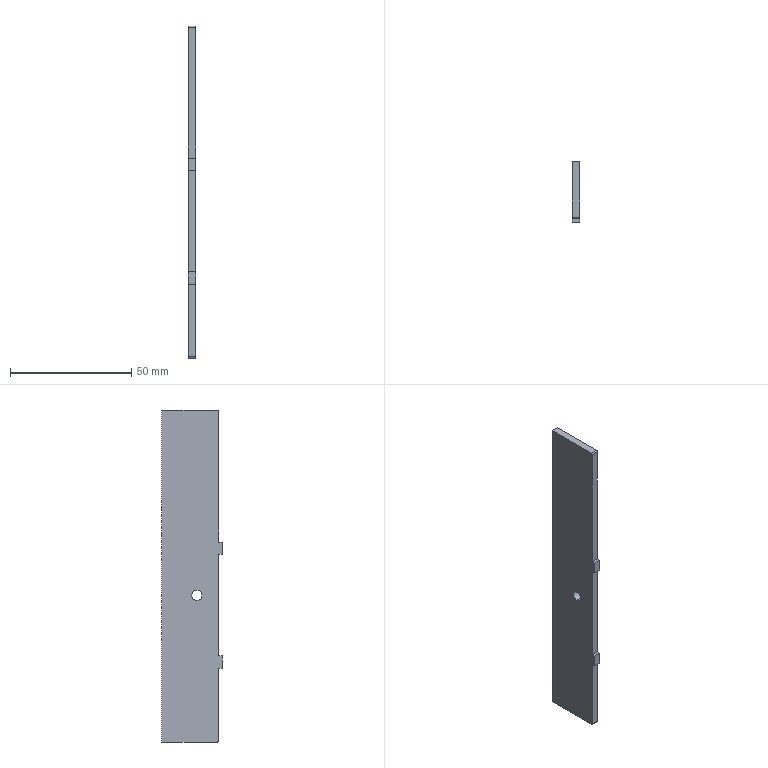Part | STEP file | HESS-408-70-15W-W-23-lower door frame support plate | 1 solid | 18 faces | box 3 x 25 x 137 mm | volume 9662 mm3 | plane 14 | cylinder 4 | commonest cylinder face diameters 1 x2 4.2 x2
STEP:
#1=CARTESIAN_POINT('',(0.,0.,0.));
#2=DIRECTION('',(0.,0.,1.));
#3=DIRECTION('',(1.,0.,0.));
#4=AXIS2_PLACEMENT_3D('',#1,#2,#3);
#5=CARTESIAN_POINT('',(-3.,-2.75,-10.1));
#6=VERTEX_POINT('',#5);
#7=CARTESIAN_POINT('',(0.,-2.75,-10.1));
#8=VERTEX_POINT('',#7);
#9=CARTESIAN_POINT('',(-10.,-2.75,-10.1));
#10=DIRECTION('',(1.,0.,0.));
#11=VECTOR('',#10,1.);
#12=LINE('',#9,#11);
#13=CARTESIAN_POINT('',(-10.,-2.75,-8.));
#14=DIRECTION('',(1.,0.,0.));
#15=DIRECTION('',(0.,0.,-1.));
#16=AXIS2_PLACEMENT_3D('',#13,#14,#15);
#17=CYLINDRICAL_SURFACE('',#16,2.1);
#18=CARTESIAN_POINT('',(6.283,0.));
#19=DIRECTION('',(0.,1.));
#20=VECTOR('',#19,1.);
#21=LINE('',#18,#20);
#22=(GEOMETRIC_REPRESENTATION_CONTEXT(2)PARAMETRIC_REPRESENTATION_CONTEXT()REPRESENTATION_CONTEXT('',''));
#23=DEFINITIONAL_REPRESENTATION('',(#21),#22);
#24=PCURVE('',#17,#23);
#25=CARTESIAN_POINT('',(-10.,-2.75,-8.));
#26=DIRECTION('',(1.,0.,0.));
#27=DIRECTION('',(0.,0.,-1.));
#28=AXIS2_PLACEMENT_3D('',#25,#26,#27);
#29=CYLINDRICAL_SURFACE('',#28,2.1);
#30=CARTESIAN_POINT('',(0.,0.));
#31=DIRECTION('',(0.,1.));
#32=VECTOR('',#31,1.);
#33=LINE('',#30,#32);
#34=(GEOMETRIC_REPRESENTATION_CONTEXT(2)PARAMETRIC_REPRESENTATION_CONTEXT()REPRESENTATION_CONTEXT('',''));
#35=DEFINITIONAL_REPRESENTATION('',(#33),#34);
#36=PCURVE('',#29,#35);
#37=SURFACE_CURVE('',#12,(#24,#36),.PCURVE_S1.);
#38=EDGE_CURVE('',#6,#8,#37,.T.);
#39=ORIENTED_EDGE('',*,*,#38,.T.);
#40=CARTESIAN_POINT('',(0.,-2.75,-5.9));
#41=VERTEX_POINT('',#40);
#42=CARTESIAN_POINT('',(0.,-2.75,-8.));
#43=DIRECTION('',(1.,0.,0.));
#44=DIRECTION('',(0.,0.,-1.));
#45=AXIS2_PLACEMENT_3D('',#42,#43,#44);
#46=CIRCLE('',#45,2.1);
#47=CARTESIAN_POINT('',(0.,10.));
#48=DIRECTION('',(1.,0.));
#49=VECTOR('',#48,1.);
#50=LINE('',#47,#49);
#51=(GEOMETRIC_REPRESENTATION_CONTEXT(2)PARAMETRIC_REPRESENTATION_CONTEXT()REPRESENTATION_CONTEXT('',''));
#52=DEFINITIONAL_REPRESENTATION('',(#50),#51);
#53=PCURVE('',#17,#52);
#54=CARTESIAN_POINT('',(0.,0.,0.));
#55=DIRECTION('',(-1.,0.,0.));
#56=DIRECTION('',(0.,0.,1.));
#57=AXIS2_PLACEMENT_3D('',#54,#55,#56);
#58=PLANE('',#57);
#59=CARTESIAN_POINT('',(-10.1,-2.75));
#60=CARTESIAN_POINT('',(-10.1,0.8873));
#61=CARTESIAN_POINT('',(-6.95,-0.9313));
#62=CARTESIAN_POINT('',(-3.8,-2.75));
#63=CARTESIAN_POINT('',(-6.95,-4.569));
#64=CARTESIAN_POINT('',(-10.1,-6.387));
#65=CARTESIAN_POINT('',(-10.1,-2.75));
#66=(BOUNDED_CURVE()B_SPLINE_CURVE(2,(#59,#60,#61,#62,#63,#64,#65),.UNSPECIFIED.,.T.,.F.)B_SPLINE_CURVE_WITH_KNOTS((1,2,2,2,2,1),(-2.094,0.,2.094,4.189,6.283,8.378),.UNSPECIFIED.)CURVE()GEOMETRIC_REPRESENTATION_ITEM()RATIONAL_B_SPLINE_CURVE((1.,0.5,1.,0.5,1.,0.5,1.))REPRESENTATION_ITEM(''));
#67=(GEOMETRIC_REPRESENTATION_CONTEXT(2)PARAMETRIC_REPRESENTATION_CONTEXT()REPRESENTATION_CONTEXT('',''));
#68=DEFINITIONAL_REPRESENTATION('',(#66),#67);
#69=PCURVE('',#58,#68);
#70=SURFACE_CURVE('',#46,(#53,#69),.PCURVE_S1.);
#71=EDGE_CURVE('',#41,#8,#70,.T.);
#72=ORIENTED_EDGE('',*,*,#71,.F.);
#73=CARTESIAN_POINT('',(-3.,-2.75,-5.9));
#74=VERTEX_POINT('',#73);
#75=CARTESIAN_POINT('',(-10.,-2.75,-5.9));
#76=DIRECTION('',(1.,0.,0.));
#77=VECTOR('',#76,1.);
#78=LINE('',#75,#77);
#79=CARTESIAN_POINT('',(3.142,0.));
#80=DIRECTION('',(0.,1.));
#81=VECTOR('',#80,1.);
#82=LINE('',#79,#81);
#83=(GEOMETRIC_REPRESENTATION_CONTEXT(2)PARAMETRIC_REPRESENTATION_CONTEXT()REPRESENTATION_CONTEXT('',''));
#84=DEFINITIONAL_REPRESENTATION('',(#82),#83);
#85=PCURVE('',#17,#84);
#86=CARTESIAN_POINT('',(3.142,0.));
#87=DIRECTION('',(0.,1.));
#88=VECTOR('',#87,1.);
#89=LINE('',#86,#88);
#90=(GEOMETRIC_REPRESENTATION_CONTEXT(2)PARAMETRIC_REPRESENTATION_CONTEXT()REPRESENTATION_CONTEXT('',''));
#91=DEFINITIONAL_REPRESENTATION('',(#89),#90);
#92=PCURVE('',#29,#91);
#93=SURFACE_CURVE('',#78,(#85,#92),.PCURVE_S1.);
#94=EDGE_CURVE('',#74,#41,#93,.T.);
#95=ORIENTED_EDGE('',*,*,#94,.F.);
#96=CARTESIAN_POINT('',(-3.,-2.75,-8.));
#97=DIRECTION('',(1.,0.,0.));
#98=DIRECTION('',(0.,0.,-1.));
#99=AXIS2_PLACEMENT_3D('',#96,#97,#98);
#100=CIRCLE('',#99,2.1);
#101=CARTESIAN_POINT('',(0.,7.));
#102=DIRECTION('',(1.,0.));
#103=VECTOR('',#102,1.);
#104=LINE('',#101,#103);
#105=(GEOMETRIC_REPRESENTATION_CONTEXT(2)PARAMETRIC_REPRESENTATION_CONTEXT()REPRESENTATION_CONTEXT('',''));
#106=DEFINITIONAL_REPRESENTATION('',(#104),#105);
#107=PCURVE('',#17,#106);
#108=CARTESIAN_POINT('',(-3.,0.,0.));
#109=DIRECTION('',(-1.,0.,0.));
#110=DIRECTION('',(0.,0.,1.));
#111=AXIS2_PLACEMENT_3D('',#108,#109,#110);
#112=PLANE('',#111);
#113=CARTESIAN_POINT('',(-10.1,-2.75));
#114=CARTESIAN_POINT('',(-10.1,0.8873));
#115=CARTESIAN_POINT('',(-6.95,-0.9313));
#116=CARTESIAN_POINT('',(-3.8,-2.75));
#117=CARTESIAN_POINT('',(-6.95,-4.569));
#118=CARTESIAN_POINT('',(-10.1,-6.387));
#119=CARTESIAN_POINT('',(-10.1,-2.75));
#120=(BOUNDED_CURVE()B_SPLINE_CURVE(2,(#113,#114,#115,#116,#117,#118,#119),.UNSPECIFIED.,.T.,.F.)B_SPLINE_CURVE_WITH_KNOTS((1,2,2,2,2,1),(-2.094,0.,2.094,4.189,6.283,8.378),.UNSPECIFIED.)CURVE()GEOMETRIC_REPRESENTATION_ITEM()RATIONAL_B_SPLINE_CURVE((1.,0.5,1.,0.5,1.,0.5,1.))REPRESENTATION_ITEM(''));
#121=(GEOMETRIC_REPRESENTATION_CONTEXT(2)PARAMETRIC_REPRESENTATION_CONTEXT()REPRESENTATION_CONTEXT('',''));
#122=DEFINITIONAL_REPRESENTATION('',(#120),#121);
#123=PCURVE('',#112,#122);
#124=SURFACE_CURVE('',#100,(#107,#123),.PCURVE_S1.);
#125=EDGE_CURVE('',#74,#6,#124,.T.);
#126=ORIENTED_EDGE('',*,*,#125,.T.);
#127=EDGE_LOOP('',(#39,#72,#95,#126));
#128=FACE_BOUND('',#127,.F.);
#129=ADVANCED_FACE('',(#128),#17,.F.);
#130=CARTESIAN_POINT('',(0.,-13.25,14.));
#131=VERTEX_POINT('',#130);
#132=CARTESIAN_POINT('',(0.,-11.75,14.));
#133=VERTEX_POINT('',#132);
#134=CARTESIAN_POINT('',(0.,-11.75,14.));
#135=DIRECTION('',(0.,1.,0.));
#136=VECTOR('',#135,1.);
#137=LINE('',#134,#136);
#138=CARTESIAN_POINT('',(14.,-11.75));
#139=DIRECTION('',(0.,1.));
#140=VECTOR('',#139,1.);
#141=LINE('',#138,#140);
#142=(GEOMETRIC_REPRESENTATION_CONTEXT(2)PARAMETRIC_REPRESENTATION_CONTEXT()REPRESENTATION_CONTEXT('',''));
#143=DEFINITIONAL_REPRESENTATION('',(#141),#142);
#144=PCURVE('',#58,#143);
#145=CARTESIAN_POINT('',(0.,-11.75,14.));
#146=DIRECTION('',(0.,0.,1.));
#147=DIRECTION('',(1.,0.,0.));
#148=AXIS2_PLACEMENT_3D('',#145,#146,#147);
#149=PLANE('',#148);
#150=CARTESIAN_POINT('',(0.,0.));
#151=DIRECTION('',(0.,1.));
#152=VECTOR('',#151,1.);
#153=LINE('',#150,#152);
#154=(GEOMETRIC_REPRESENTATION_CONTEXT(2)PARAMETRIC_REPRESENTATION_CONTEXT()REPRESENTATION_CONTEXT('',''));
#155=DEFINITIONAL_REPRESENTATION('',(#153),#154);
#156=PCURVE('',#149,#155);
#157=SURFACE_CURVE('',#137,(#144,#156),.PCURVE_S1.);
#158=EDGE_CURVE('',#131,#133,#157,.T.);
#159=ORIENTED_EDGE('',*,*,#158,.F.);
#160=CARTESIAN_POINT('',(0.,-13.25,9.));
#161=VERTEX_POINT('',#160);
#162=CARTESIAN_POINT('',(0.,-13.25,0.));
#163=DIRECTION('',(0.,0.,1.));
#164=VECTOR('',#163,1.);
#165=LINE('',#162,#164);
#166=CARTESIAN_POINT('',(0.,-13.25));
#167=DIRECTION('',(1.,0.));
#168=VECTOR('',#167,1.);
#169=LINE('',#166,#168);
#170=(GEOMETRIC_REPRESENTATION_CONTEXT(2)PARAMETRIC_REPRESENTATION_CONTEXT()REPRESENTATION_CONTEXT('',''));
#171=DEFINITIONAL_REPRESENTATION('',(#169),#170);
#172=PCURVE('',#58,#171);
#173=CARTESIAN_POINT('',(0.,-13.25,9.));
#174=DIRECTION('',(0.,-1.,0.));
#175=DIRECTION('',(0.,0.,-1.));
#176=AXIS2_PLACEMENT_3D('',#173,#174,#175);
#177=PLANE('',#176);
#178=CARTESIAN_POINT('',(9.,0.));
#179=DIRECTION('',(-1.,0.));
#180=VECTOR('',#179,1.);
#181=LINE('',#178,#180);
#182=(GEOMETRIC_REPRESENTATION_CONTEXT(2)PARAMETRIC_REPRESENTATION_CONTEXT()REPRESENTATION_CONTEXT('',''));
#183=DEFINITIONAL_REPRESENTATION('',(#181),#182);
#184=PCURVE('',#177,#183);
#185=SURFACE_CURVE('',#165,(#172,#184),.PCURVE_S1.);
#186=EDGE_CURVE('',#161,#131,#185,.T.);
#187=ORIENTED_EDGE('',*,*,#186,.F.);
#188=CARTESIAN_POINT('',(0.,-11.75,9.));
#189=VERTEX_POINT('',#188);
#190=CARTESIAN_POINT('',(0.,-11.75,9.));
#191=DIRECTION('',(0.,-1.,0.));
#192=VECTOR('',#191,1.);
#193=LINE('',#190,#192);
#194=CARTESIAN_POINT('',(9.,-11.75));
#195=DIRECTION('',(0.,-1.));
#196=VECTOR('',#195,1.);
#197=LINE('',#194,#196);
#198=(GEOMETRIC_REPRESENTATION_CONTEXT(2)PARAMETRIC_REPRESENTATION_CONTEXT()REPRESENTATION_CONTEXT('',''));
#199=DEFINITIONAL_REPRESENTATION('',(#197),#198);
#200=PCURVE('',#58,#199);
#201=CARTESIAN_POINT('',(0.,-11.75,9.));
#202=DIRECTION('',(0.,0.,-1.));
#203=DIRECTION('',(-1.,0.,0.));
#204=AXIS2_PLACEMENT_3D('',#201,#202,#203);
#205=PLANE('',#204);
#206=CARTESIAN_POINT('',(0.,0.));
#207=DIRECTION('',(0.,-1.));
#208=VECTOR('',#207,1.);
#209=LINE('',#206,#208);
#210=(GEOMETRIC_REPRESENTATION_CONTEXT(2)PARAMETRIC_REPRESENTATION_CONTEXT()REPRESENTATION_CONTEXT('',''));
#211=DEFINITIONAL_REPRESENTATION('',(#209),#210);
#212=PCURVE('',#205,#211);
#213=SURFACE_CURVE('',#193,(#200,#212),.PCURVE_S1.);
#214=EDGE_CURVE('',#189,#161,#213,.T.);
#215=ORIENTED_EDGE('',*,*,#214,.F.);
#216=CARTESIAN_POINT('',(0.,-11.75,-33.));
#217=VERTEX_POINT('',#216);
#218=CARTESIAN_POINT('',(0.,-11.75,0.));
#219=DIRECTION('',(0.,0.,1.));
#220=VECTOR('',#219,1.);
#221=LINE('',#218,#220);
#222=CARTESIAN_POINT('',(0.,-11.75));
#223=DIRECTION('',(1.,0.));
#224=VECTOR('',#223,1.);
#225=LINE('',#222,#224);
#226=(GEOMETRIC_REPRESENTATION_CONTEXT(2)PARAMETRIC_REPRESENTATION_CONTEXT()REPRESENTATION_CONTEXT('',''));
#227=DEFINITIONAL_REPRESENTATION('',(#225),#226);
#228=PCURVE('',#58,#227);
#229=CARTESIAN_POINT('',(-3.,-11.75,68.5));
#230=DIRECTION('',(0.,-1.,0.));
#231=DIRECTION('',(0.,0.,-1.));
#232=AXIS2_PLACEMENT_3D('',#229,#230,#231);
#233=PLANE('',#232);
#234=CARTESIAN_POINT('',(68.5,3.));
#235=DIRECTION('',(-1.,0.));
#236=VECTOR('',#235,1.);
#237=LINE('',#234,#236);
#238=(GEOMETRIC_REPRESENTATION_CONTEXT(2)PARAMETRIC_REPRESENTATION_CONTEXT()REPRESENTATION_CONTEXT('',''));
#239=DEFINITIONAL_REPRESENTATION('',(#237),#238);
#240=PCURVE('',#233,#239);
#241=SURFACE_CURVE('',#221,(#228,#240),.PCURVE_S1.);
#242=EDGE_CURVE('',#217,#189,#241,.T.);
#243=ORIENTED_EDGE('',*,*,#242,.F.);
#244=CARTESIAN_POINT('',(0.,-13.25,-33.));
#245=VERTEX_POINT('',#244);
#246=CARTESIAN_POINT('',(0.,-11.75,-33.));
#247=DIRECTION('',(0.,1.,0.));
#248=VECTOR('',#247,1.);
#249=LINE('',#246,#248);
#250=CARTESIAN_POINT('',(-33.,-11.75));
#251=DIRECTION('',(0.,1.));
#252=VECTOR('',#251,1.);
#253=LINE('',#250,#252);
#254=(GEOMETRIC_REPRESENTATION_CONTEXT(2)PARAMETRIC_REPRESENTATION_CONTEXT()REPRESENTATION_CONTEXT('',''));
#255=DEFINITIONAL_REPRESENTATION('',(#253),#254);
#256=PCURVE('',#58,#255);
#257=CARTESIAN_POINT('',(0.,-11.75,-33.));
#258=DIRECTION('',(0.,0.,1.));
#259=DIRECTION('',(1.,0.,0.));
#260=AXIS2_PLACEMENT_3D('',#257,#258,#259);
#261=PLANE('',#260);
#262=CARTESIAN_POINT('',(0.,0.));
#263=DIRECTION('',(0.,1.));
#264=VECTOR('',#263,1.);
#265=LINE('',#262,#264);
#266=(GEOMETRIC_REPRESENTATION_CONTEXT(2)PARAMETRIC_REPRESENTATION_CONTEXT()REPRESENTATION_CONTEXT('',''));
#267=DEFINITIONAL_REPRESENTATION('',(#265),#266);
#268=PCURVE('',#261,#267);
#269=SURFACE_CURVE('',#249,(#256,#268),.PCURVE_S1.);
#270=EDGE_CURVE('',#245,#217,#269,.T.);
#271=ORIENTED_EDGE('',*,*,#270,.F.);
#272=CARTESIAN_POINT('',(0.,-13.25,-38.));
#273=VERTEX_POINT('',#272);
#274=CARTESIAN_POINT('',(0.,-13.25,0.));
#275=DIRECTION('',(0.,0.,1.));
#276=VECTOR('',#275,1.);
#277=LINE('',#274,#276);
#278=CARTESIAN_POINT('',(0.,-13.25));
#279=DIRECTION('',(1.,0.));
#280=VECTOR('',#279,1.);
#281=LINE('',#278,#280);
#282=(GEOMETRIC_REPRESENTATION_CONTEXT(2)PARAMETRIC_REPRESENTATION_CONTEXT()REPRESENTATION_CONTEXT('',''));
#283=DEFINITIONAL_REPRESENTATION('',(#281),#282);
#284=PCURVE('',#58,#283);
#285=CARTESIAN_POINT('',(0.,-13.25,-38.));
#286=DIRECTION('',(0.,-1.,0.));
#287=DIRECTION('',(0.,0.,-1.));
#288=AXIS2_PLACEMENT_3D('',#285,#286,#287);
#289=PLANE('',#288);
#290=CARTESIAN_POINT('',(-38.,0.));
#291=DIRECTION('',(-1.,0.));
#292=VECTOR('',#291,1.);
#293=LINE('',#290,#292);
#294=(GEOMETRIC_REPRESENTATION_CONTEXT(2)PARAMETRIC_REPRESENTATION_CONTEXT()REPRESENTATION_CONTEXT('',''));
#295=DEFINITIONAL_REPRESENTATION('',(#293),#294);
#296=PCURVE('',#289,#295);
#297=SURFACE_CURVE('',#277,(#284,#296),.PCURVE_S1.);
#298=EDGE_CURVE('',#273,#245,#297,.T.);
#299=ORIENTED_EDGE('',*,*,#298,.F.);
#300=CARTESIAN_POINT('',(0.,-11.75,-38.));
#301=VERTEX_POINT('',#300);
#302=CARTESIAN_POINT('',(0.,-11.75,-38.));
#303=DIRECTION('',(0.,-1.,0.));
#304=VECTOR('',#303,1.);
#305=LINE('',#302,#304);
#306=CARTESIAN_POINT('',(-38.,-11.75));
#307=DIRECTION('',(0.,-1.));
#308=VECTOR('',#307,1.);
#309=LINE('',#306,#308);
#310=(GEOMETRIC_REPRESENTATION_CONTEXT(2)PARAMETRIC_REPRESENTATION_CONTEXT()REPRESENTATION_CONTEXT('',''));
#311=DEFINITIONAL_REPRESENTATION('',(#309),#310);
#312=PCURVE('',#58,#311);
#313=CARTESIAN_POINT('',(0.,-11.75,-38.));
#314=DIRECTION('',(0.,0.,-1.));
#315=DIRECTION('',(-1.,0.,0.));
#316=AXIS2_PLACEMENT_3D('',#313,#314,#315);
#317=PLANE('',#316);
#318=CARTESIAN_POINT('',(0.,0.));
#319=DIRECTION('',(0.,-1.));
#320=VECTOR('',#319,1.);
#321=LINE('',#318,#320);
#322=(GEOMETRIC_REPRESENTATION_CONTEXT(2)PARAMETRIC_REPRESENTATION_CONTEXT()REPRESENTATION_CONTEXT('',''));
#323=DEFINITIONAL_REPRESENTATION('',(#321),#322);
#324=PCURVE('',#317,#323);
#325=SURFACE_CURVE('',#305,(#312,#324),.PCURVE_S1.);
#326=EDGE_CURVE('',#301,#273,#325,.T.);
#327=ORIENTED_EDGE('',*,*,#326,.F.);
#328=CARTESIAN_POINT('',(0.,-11.75,-68.));
#329=VERTEX_POINT('',#328);
#330=CARTESIAN_POINT('',(0.,-11.75,0.));
#331=DIRECTION('',(0.,0.,1.));
#332=VECTOR('',#331,1.);
#333=LINE('',#330,#332);
#334=CARTESIAN_POINT('',(0.,-11.75));
#335=DIRECTION('',(1.,0.));
#336=VECTOR('',#335,1.);
#337=LINE('',#334,#336);
#338=(GEOMETRIC_REPRESENTATION_CONTEXT(2)PARAMETRIC_REPRESENTATION_CONTEXT()REPRESENTATION_CONTEXT('',''));
#339=DEFINITIONAL_REPRESENTATION('',(#337),#338);
#340=PCURVE('',#58,#339);
#341=CARTESIAN_POINT('',(-3.,-11.75,68.5));
#342=DIRECTION('',(0.,-1.,0.));
#343=DIRECTION('',(0.,0.,-1.));
#344=AXIS2_PLACEMENT_3D('',#341,#342,#343);
#345=PLANE('',#344);
#346=CARTESIAN_POINT('',(68.5,3.));
#347=DIRECTION('',(-1.,0.));
#348=VECTOR('',#347,1.);
#349=LINE('',#346,#348);
#350=(GEOMETRIC_REPRESENTATION_CONTEXT(2)PARAMETRIC_REPRESENTATION_CONTEXT()REPRESENTATION_CONTEXT('',''));
#351=DEFINITIONAL_REPRESENTATION('',(#349),#350);
#352=PCURVE('',#345,#351);
#353=SURFACE_CURVE('',#333,(#340,#352),.PCURVE_S1.);
#354=EDGE_CURVE('',#329,#301,#353,.T.);
#355=ORIENTED_EDGE('',*,*,#354,.F.);
#356=CARTESIAN_POINT('',(0.,-11.25,-68.5));
#357=VERTEX_POINT('',#356);
#358=CARTESIAN_POINT('',(0.,-11.25,-68.));
#359=DIRECTION('',(-1.,0.,0.));
#360=DIRECTION('',(0.,0.,-1.));
#361=AXIS2_PLACEMENT_3D('',#358,#359,#360);
#362=CIRCLE('',#361,0.5);
#363=CARTESIAN_POINT('',(-68.,-11.25));
#364=DIRECTION('',(-1.,0.));
#365=AXIS2_PLACEMENT_2D('',#363,#364);
#366=CIRCLE('',#365,0.5);
#367=(GEOMETRIC_REPRESENTATION_CONTEXT(2)PARAMETRIC_REPRESENTATION_CONTEXT()REPRESENTATION_CONTEXT('',''));
#368=DEFINITIONAL_REPRESENTATION('',(#366),#367);
#369=PCURVE('',#58,#368);
#370=CARTESIAN_POINT('',(-3.,-11.25,-68.));
#371=DIRECTION('',(1.,0.,0.));
#372=DIRECTION('',(0.,0.,-1.));
#373=AXIS2_PLACEMENT_3D('',#370,#371,#372);
#374=CYLINDRICAL_SURFACE('',#373,0.5);
#375=CARTESIAN_POINT('',(6.283,3.));
#376=DIRECTION('',(-1.,0.));
#377=VECTOR('',#376,1.);
#378=LINE('',#375,#377);
#379=(GEOMETRIC_REPRESENTATION_CONTEXT(2)PARAMETRIC_REPRESENTATION_CONTEXT()REPRESENTATION_CONTEXT('',''));
#380=DEFINITIONAL_REPRESENTATION('',(#378),#379);
#381=PCURVE('',#374,#380);
#382=SURFACE_CURVE('',#362,(#369,#381),.PCURVE_S1.);
#383=EDGE_CURVE('',#357,#329,#382,.T.);
#384=ORIENTED_EDGE('',*,*,#383,.F.);
#385=CARTESIAN_POINT('',(0.,11.75,-68.5));
#386=VERTEX_POINT('',#385);
#387=CARTESIAN_POINT('',(0.,0.,-68.5));
#388=DIRECTION('',(0.,-1.,0.));
#389=VECTOR('',#388,1.);
#390=LINE('',#387,#389);
#391=CARTESIAN_POINT('',(-68.5,0.));
#392=DIRECTION('',(0.,-1.));
#393=VECTOR('',#392,1.);
#394=LINE('',#391,#393);
#395=(GEOMETRIC_REPRESENTATION_CONTEXT(2)PARAMETRIC_REPRESENTATION_CONTEXT()REPRESENTATION_CONTEXT('',''));
#396=DEFINITIONAL_REPRESENTATION('',(#394),#395);
#397=PCURVE('',#58,#396);
#398=CARTESIAN_POINT('',(-3.,-11.75,-68.5));
#399=DIRECTION('',(0.,0.,-1.));
#400=DIRECTION('',(-1.,0.,0.));
#401=AXIS2_PLACEMENT_3D('',#398,#399,#400);
#402=PLANE('',#401);
#403=CARTESIAN_POINT('',(-3.,11.75));
#404=DIRECTION('',(0.,-1.));
#405=VECTOR('',#404,1.);
#406=LINE('',#403,#405);
#407=(GEOMETRIC_REPRESENTATION_CONTEXT(2)PARAMETRIC_REPRESENTATION_CONTEXT()REPRESENTATION_CONTEXT('',''));
#408=DEFINITIONAL_REPRESENTATION('',(#406),#407);
#409=PCURVE('',#402,#408);
#410=SURFACE_CURVE('',#390,(#397,#409),.PCURVE_S1.);
#411=EDGE_CURVE('',#386,#357,#410,.T.);
#412=ORIENTED_EDGE('',*,*,#411,.F.);
#413=CARTESIAN_POINT('',(0.,11.75,68.5));
#414=VERTEX_POINT('',#413);
#415=CARTESIAN_POINT('',(0.,11.75,0.));
#416=DIRECTION('',(0.,0.,-1.));
#417=VECTOR('',#416,1.);
#418=LINE('',#415,#417);
#419=CARTESIAN_POINT('',(0.,11.75));
#420=DIRECTION('',(-1.,0.));
#421=VECTOR('',#420,1.);
#422=LINE('',#419,#421);
#423=(GEOMETRIC_REPRESENTATION_CONTEXT(2)PARAMETRIC_REPRESENTATION_CONTEXT()REPRESENTATION_CONTEXT('',''));
#424=DEFINITIONAL_REPRESENTATION('',(#422),#423);
#425=PCURVE('',#58,#424);
#426=CARTESIAN_POINT('',(-3.,11.75,68.5));
#427=DIRECTION('',(0.,1.,0.));
#428=DIRECTION('',(0.,0.,1.));
#429=AXIS2_PLACEMENT_3D('',#426,#427,#428);
#430=PLANE('',#429);
#431=CARTESIAN_POINT('',(-68.5,3.));
#432=DIRECTION('',(-1.,0.));
#433=VECTOR('',#432,1.);
#434=LINE('',#431,#433);
#435=(GEOMETRIC_REPRESENTATION_CONTEXT(2)PARAMETRIC_REPRESENTATION_CONTEXT()REPRESENTATION_CONTEXT('',''));
#436=DEFINITIONAL_REPRESENTATION('',(#434),#435);
#437=PCURVE('',#430,#436);
#438=SURFACE_CURVE('',#418,(#425,#437),.PCURVE_S1.);
#439=EDGE_CURVE('',#414,#386,#438,.T.);
#440=ORIENTED_EDGE('',*,*,#439,.F.);
#441=CARTESIAN_POINT('',(0.,-11.25,68.5));
#442=VERTEX_POINT('',#441);
#443=CARTESIAN_POINT('',(0.,0.,68.5));
#444=DIRECTION('',(0.,1.,0.));
#445=VECTOR('',#444,1.);
#446=LINE('',#443,#445);
#447=CARTESIAN_POINT('',(68.5,0.));
#448=DIRECTION('',(0.,1.));
#449=VECTOR('',#448,1.);
#450=LINE('',#447,#449);
#451=(GEOMETRIC_REPRESENTATION_CONTEXT(2)PARAMETRIC_REPRESENTATION_CONTEXT()REPRESENTATION_CONTEXT('',''));
#452=DEFINITIONAL_REPRESENTATION('',(#450),#451);
#453=PCURVE('',#58,#452);
#454=CARTESIAN_POINT('',(-3.,-11.75,68.5));
#455=DIRECTION('',(0.,0.,1.));
#456=DIRECTION('',(1.,0.,0.));
#457=AXIS2_PLACEMENT_3D('',#454,#455,#456);
#458=PLANE('',#457);
#459=CARTESIAN_POINT('',(3.,11.75));
#460=DIRECTION('',(0.,1.));
#461=VECTOR('',#460,1.);
#462=LINE('',#459,#461);
#463=(GEOMETRIC_REPRESENTATION_CONTEXT(2)PARAMETRIC_REPRESENTATION_CONTEXT()REPRESENTATION_CONTEXT('',''));
#464=DEFINITIONAL_REPRESENTATION('',(#462),#463);
#465=PCURVE('',#458,#464);
#466=SURFACE_CURVE('',#446,(#453,#465),.PCURVE_S1.);
#467=EDGE_CURVE('',#442,#414,#466,.T.);
#468=ORIENTED_EDGE('',*,*,#467,.F.);
#469=CARTESIAN_POINT('',(0.,-11.75,68.));
#470=VERTEX_POINT('',#469);
#471=CARTESIAN_POINT('',(0.,-11.25,68.));
#472=DIRECTION('',(-1.,0.,0.));
#473=DIRECTION('',(0.,0.,-1.));
#474=AXIS2_PLACEMENT_3D('',#471,#472,#473);
#475=CIRCLE('',#474,0.5);
#476=CARTESIAN_POINT('',(68.,-11.25));
#477=DIRECTION('',(-1.,0.));
#478=AXIS2_PLACEMENT_2D('',#476,#477);
#479=CIRCLE('',#478,0.5);
#480=(GEOMETRIC_REPRESENTATION_CONTEXT(2)PARAMETRIC_REPRESENTATION_CONTEXT()REPRESENTATION_CONTEXT('',''));
#481=DEFINITIONAL_REPRESENTATION('',(#479),#480);
#482=PCURVE('',#58,#481);
#483=CARTESIAN_POINT('',(-3.,-11.25,68.));
#484=DIRECTION('',(1.,0.,0.));
#485=DIRECTION('',(0.,0.,-1.));
#486=AXIS2_PLACEMENT_3D('',#483,#484,#485);
#487=CYLINDRICAL_SURFACE('',#486,0.5);
#488=CARTESIAN_POINT('',(6.283,3.));
#489=DIRECTION('',(-1.,0.));
#490=VECTOR('',#489,1.);
#491=LINE('',#488,#490);
#492=(GEOMETRIC_REPRESENTATION_CONTEXT(2)PARAMETRIC_REPRESENTATION_CONTEXT()REPRESENTATION_CONTEXT('',''));
#493=DEFINITIONAL_REPRESENTATION('',(#491),#492);
#494=PCURVE('',#487,#493);
#495=SURFACE_CURVE('',#475,(#482,#494),.PCURVE_S1.);
#496=EDGE_CURVE('',#470,#442,#495,.T.);
#497=ORIENTED_EDGE('',*,*,#496,.F.);
#498=CARTESIAN_POINT('',(0.,-11.75,0.));
#499=DIRECTION('',(0.,0.,1.));
#500=VECTOR('',#499,1.);
#501=LINE('',#498,#500);
#502=CARTESIAN_POINT('',(0.,-11.75));
#503=DIRECTION('',(1.,0.));
#504=VECTOR('',#503,1.);
#505=LINE('',#502,#504);
#506=(GEOMETRIC_REPRESENTATION_CONTEXT(2)PARAMETRIC_REPRESENTATION_CONTEXT()REPRESENTATION_CONTEXT('',''));
#507=DEFINITIONAL_REPRESENTATION('',(#505),#506);
#508=PCURVE('',#58,#507);
#509=CARTESIAN_POINT('',(-3.,-11.75,68.5));
#510=DIRECTION('',(0.,-1.,0.));
#511=DIRECTION('',(0.,0.,-1.));
#512=AXIS2_PLACEMENT_3D('',#509,#510,#511);
#513=PLANE('',#512);
#514=CARTESIAN_POINT('',(68.5,3.));
#515=DIRECTION('',(-1.,0.));
#516=VECTOR('',#515,1.);
#517=LINE('',#514,#516);
#518=(GEOMETRIC_REPRESENTATION_CONTEXT(2)PARAMETRIC_REPRESENTATION_CONTEXT()REPRESENTATION_CONTEXT('',''));
#519=DEFINITIONAL_REPRESENTATION('',(#517),#518);
#520=PCURVE('',#513,#519);
#521=SURFACE_CURVE('',#501,(#508,#520),.PCURVE_S1.);
#522=EDGE_CURVE('',#133,#470,#521,.T.);
#523=ORIENTED_EDGE('',*,*,#522,.F.);
#524=EDGE_LOOP('',(#159,#187,#215,#243,#271,#299,#327,#355,#384,#412,#440,#468,#497,#523));
#525=FACE_BOUND('',#524,.T.);
#526=CARTESIAN_POINT('',(0.,-2.75,-8.));
#527=DIRECTION('',(1.,0.,0.));
#528=DIRECTION('',(0.,0.,-1.));
#529=AXIS2_PLACEMENT_3D('',#526,#527,#528);
#530=CIRCLE('',#529,2.1);
#531=CARTESIAN_POINT('',(-10.1,-2.75));
#532=CARTESIAN_POINT('',(-10.1,0.8873));
#533=CARTESIAN_POINT('',(-6.95,-0.9313));
#534=CARTESIAN_POINT('',(-3.8,-2.75));
#535=CARTESIAN_POINT('',(-6.95,-4.569));
#536=CARTESIAN_POINT('',(-10.1,-6.387));
#537=CARTESIAN_POINT('',(-10.1,-2.75));
#538=(BOUNDED_CURVE()B_SPLINE_CURVE(2,(#531,#532,#533,#534,#535,#536,#537),.UNSPECIFIED.,.T.,.F.)B_SPLINE_CURVE_WITH_KNOTS((1,2,2,2,2,1),(-2.094,0.,2.094,4.189,6.283,8.378),.UNSPECIFIED.)CURVE()GEOMETRIC_REPRESENTATION_ITEM()RATIONAL_B_SPLINE_CURVE((1.,0.5,1.,0.5,1.,0.5,1.))REPRESENTATION_ITEM(''));
#539=(GEOMETRIC_REPRESENTATION_CONTEXT(2)PARAMETRIC_REPRESENTATION_CONTEXT()REPRESENTATION_CONTEXT('',''));
#540=DEFINITIONAL_REPRESENTATION('',(#538),#539);
#541=PCURVE('',#58,#540);
#542=CARTESIAN_POINT('',(0.,10.));
#543=DIRECTION('',(1.,0.));
#544=VECTOR('',#543,1.);
#545=LINE('',#542,#544);
#546=(GEOMETRIC_REPRESENTATION_CONTEXT(2)PARAMETRIC_REPRESENTATION_CONTEXT()REPRESENTATION_CONTEXT('',''));
#547=DEFINITIONAL_REPRESENTATION('',(#545),#546);
#548=PCURVE('',#29,#547);
#549=SURFACE_CURVE('',#530,(#541,#548),.PCURVE_S1.);
#550=EDGE_CURVE('',#8,#41,#549,.T.);
#551=ORIENTED_EDGE('',*,*,#550,.F.);
#552=ORIENTED_EDGE('',*,*,#71,.F.);
#553=EDGE_LOOP('',(#551,#552));
#554=FACE_BOUND('',#553,.T.);
#555=ADVANCED_FACE('',(#525,#554),#58,.F.);
#556=CARTESIAN_POINT('',(-3.,-11.75,68.));
#557=VERTEX_POINT('',#556);
#558=CARTESIAN_POINT('',(-3.,-11.75,68.));
#559=DIRECTION('',(-1.,0.,0.));
#560=VECTOR('',#559,1.);
#561=LINE('',#558,#560);
#562=CARTESIAN_POINT('',(0.5,0.));
#563=DIRECTION('',(0.,-1.));
#564=VECTOR('',#563,1.);
#565=LINE('',#562,#564);
#566=(GEOMETRIC_REPRESENTATION_CONTEXT(2)PARAMETRIC_REPRESENTATION_CONTEXT()REPRESENTATION_CONTEXT('',''));
#567=DEFINITIONAL_REPRESENTATION('',(#565),#566);
#568=PCURVE('',#513,#567);
#569=CARTESIAN_POINT('',(4.712,0.));
#570=DIRECTION('',(0.,-1.));
#571=VECTOR('',#570,1.);
#572=LINE('',#569,#571);
#573=(GEOMETRIC_REPRESENTATION_CONTEXT(2)PARAMETRIC_REPRESENTATION_CONTEXT()REPRESENTATION_CONTEXT('',''));
#574=DEFINITIONAL_REPRESENTATION('',(#572),#573);
#575=PCURVE('',#487,#574);
#576=SURFACE_CURVE('',#561,(#568,#575),.PCURVE_S1.);
#577=EDGE_CURVE('',#470,#557,#576,.T.);
#578=ORIENTED_EDGE('',*,*,#577,.T.);
#579=CARTESIAN_POINT('',(-3.,-11.75,14.));
#580=VERTEX_POINT('',#579);
#581=CARTESIAN_POINT('',(-3.,-11.75,68.5));
#582=DIRECTION('',(0.,0.,-1.));
#583=VECTOR('',#582,1.);
#584=LINE('',#581,#583);
#585=CARTESIAN_POINT('',(0.,0.));
#586=DIRECTION('',(1.,0.));
#587=VECTOR('',#586,1.);
#588=LINE('',#585,#587);
#589=(GEOMETRIC_REPRESENTATION_CONTEXT(2)PARAMETRIC_REPRESENTATION_CONTEXT()REPRESENTATION_CONTEXT('',''));
#590=DEFINITIONAL_REPRESENTATION('',(#588),#589);
#591=PCURVE('',#513,#590);
#592=CARTESIAN_POINT('',(68.5,-11.75));
#593=DIRECTION('',(-1.,0.));
#594=VECTOR('',#593,1.);
#595=LINE('',#592,#594);
#596=(GEOMETRIC_REPRESENTATION_CONTEXT(2)PARAMETRIC_REPRESENTATION_CONTEXT()REPRESENTATION_CONTEXT('',''));
#597=DEFINITIONAL_REPRESENTATION('',(#595),#596);
#598=PCURVE('',#112,#597);
#599=SURFACE_CURVE('',#584,(#591,#598),.PCURVE_S1.);
#600=EDGE_CURVE('',#557,#580,#599,.T.);
#601=ORIENTED_EDGE('',*,*,#600,.T.);
#602=CARTESIAN_POINT('',(-3.,-11.75,14.));
#603=DIRECTION('',(1.,0.,0.));
#604=VECTOR('',#603,1.);
#605=LINE('',#602,#604);
#606=CARTESIAN_POINT('',(54.5,0.));
#607=DIRECTION('',(0.,1.));
#608=VECTOR('',#607,1.);
#609=LINE('',#606,#608);
#610=(GEOMETRIC_REPRESENTATION_CONTEXT(2)PARAMETRIC_REPRESENTATION_CONTEXT()REPRESENTATION_CONTEXT('',''));
#611=DEFINITIONAL_REPRESENTATION('',(#609),#610);
#612=PCURVE('',#513,#611);
#613=CARTESIAN_POINT('',(-3.,0.));
#614=DIRECTION('',(1.,0.));
#615=VECTOR('',#614,1.);
#616=LINE('',#613,#615);
#617=(GEOMETRIC_REPRESENTATION_CONTEXT(2)PARAMETRIC_REPRESENTATION_CONTEXT()REPRESENTATION_CONTEXT('',''));
#618=DEFINITIONAL_REPRESENTATION('',(#616),#617);
#619=PCURVE('',#149,#618);
#620=SURFACE_CURVE('',#605,(#612,#619),.PCURVE_S1.);
#621=EDGE_CURVE('',#580,#133,#620,.T.);
#622=ORIENTED_EDGE('',*,*,#621,.T.);
#623=ORIENTED_EDGE('',*,*,#522,.T.);
#624=EDGE_LOOP('',(#578,#601,#622,#623));
#625=FACE_BOUND('',#624,.T.);
#626=ADVANCED_FACE('',(#625),#513,.T.);
#627=ORIENTED_EDGE('',*,*,#186,.T.);
#628=CARTESIAN_POINT('',(-3.,-13.25,14.));
#629=VERTEX_POINT('',#628);
#630=CARTESIAN_POINT('',(0.,-13.25,14.));
#631=DIRECTION('',(-1.,0.,0.));
#632=VECTOR('',#631,1.);
#633=LINE('',#630,#632);
#634=CARTESIAN_POINT('',(-5.,0.));
#635=DIRECTION('',(0.,-1.));
#636=VECTOR('',#635,1.);
#637=LINE('',#634,#636);
#638=(GEOMETRIC_REPRESENTATION_CONTEXT(2)PARAMETRIC_REPRESENTATION_CONTEXT()REPRESENTATION_CONTEXT('',''));
#639=DEFINITIONAL_REPRESENTATION('',(#637),#638);
#640=PCURVE('',#177,#639);
#641=CARTESIAN_POINT('',(0.,-1.5));
#642=DIRECTION('',(-1.,0.));
#643=VECTOR('',#642,1.);
#644=LINE('',#641,#643);
#645=(GEOMETRIC_REPRESENTATION_CONTEXT(2)PARAMETRIC_REPRESENTATION_CONTEXT()REPRESENTATION_CONTEXT('',''));
#646=DEFINITIONAL_REPRESENTATION('',(#644),#645);
#647=PCURVE('',#149,#646);
#648=SURFACE_CURVE('',#633,(#640,#647),.PCURVE_S1.);
#649=EDGE_CURVE('',#131,#629,#648,.T.);
#650=ORIENTED_EDGE('',*,*,#649,.T.);
#651=CARTESIAN_POINT('',(-3.,-13.25,9.));
#652=VERTEX_POINT('',#651);
#653=CARTESIAN_POINT('',(-3.,-13.25,9.));
#654=DIRECTION('',(0.,0.,-1.));
#655=VECTOR('',#654,1.);
#656=LINE('',#653,#655);
#657=CARTESIAN_POINT('',(0.,-3.));
#658=DIRECTION('',(1.,0.));
#659=VECTOR('',#658,1.);
#660=LINE('',#657,#659);
#661=(GEOMETRIC_REPRESENTATION_CONTEXT(2)PARAMETRIC_REPRESENTATION_CONTEXT()REPRESENTATION_CONTEXT('',''));
#662=DEFINITIONAL_REPRESENTATION('',(#660),#661);
#663=PCURVE('',#177,#662);
#664=CARTESIAN_POINT('',(9.,-13.25));
#665=DIRECTION('',(-1.,0.));
#666=VECTOR('',#665,1.);
#667=LINE('',#664,#666);
#668=(GEOMETRIC_REPRESENTATION_CONTEXT(2)PARAMETRIC_REPRESENTATION_CONTEXT()REPRESENTATION_CONTEXT('',''));
#669=DEFINITIONAL_REPRESENTATION('',(#667),#668);
#670=PCURVE('',#112,#669);
#671=SURFACE_CURVE('',#656,(#663,#670),.PCURVE_S1.);
#672=EDGE_CURVE('',#629,#652,#671,.T.);
#673=ORIENTED_EDGE('',*,*,#672,.T.);
#674=CARTESIAN_POINT('',(0.,-13.25,9.));
#675=DIRECTION('',(1.,0.,0.));
#676=VECTOR('',#675,1.);
#677=LINE('',#674,#676);
#678=CARTESIAN_POINT('',(0.,0.));
#679=DIRECTION('',(0.,1.));
#680=VECTOR('',#679,1.);
#681=LINE('',#678,#680);
#682=(GEOMETRIC_REPRESENTATION_CONTEXT(2)PARAMETRIC_REPRESENTATION_CONTEXT()REPRESENTATION_CONTEXT('',''));
#683=DEFINITIONAL_REPRESENTATION('',(#681),#682);
#684=PCURVE('',#177,#683);
#685=CARTESIAN_POINT('',(0.,-1.5));
#686=DIRECTION('',(-1.,0.));
#687=VECTOR('',#686,1.);
#688=LINE('',#685,#687);
#689=(GEOMETRIC_REPRESENTATION_CONTEXT(2)PARAMETRIC_REPRESENTATION_CONTEXT()REPRESENTATION_CONTEXT('',''));
#690=DEFINITIONAL_REPRESENTATION('',(#688),#689);
#691=PCURVE('',#205,#690);
#692=SURFACE_CURVE('',#677,(#684,#691),.PCURVE_S1.);
#693=EDGE_CURVE('',#652,#161,#692,.T.);
#694=ORIENTED_EDGE('',*,*,#693,.T.);
#695=EDGE_LOOP('',(#627,#650,#673,#694));
#696=FACE_BOUND('',#695,.T.);
#697=ADVANCED_FACE('',(#696),#177,.T.);
#698=CARTESIAN_POINT('',(-3.,-11.75,-33.));
#699=VERTEX_POINT('',#698);
#700=CARTESIAN_POINT('',(-3.,-11.75,-33.));
#701=DIRECTION('',(1.,0.,0.));
#702=VECTOR('',#701,1.);
#703=LINE('',#700,#702);
#704=CARTESIAN_POINT('',(101.5,0.));
#705=DIRECTION('',(0.,1.));
#706=VECTOR('',#705,1.);
#707=LINE('',#704,#706);
#708=(GEOMETRIC_REPRESENTATION_CONTEXT(2)PARAMETRIC_REPRESENTATION_CONTEXT()REPRESENTATION_CONTEXT('',''));
#709=DEFINITIONAL_REPRESENTATION('',(#707),#708);
#710=PCURVE('',#233,#709);
#711=CARTESIAN_POINT('',(-3.,0.));
#712=DIRECTION('',(1.,0.));
#713=VECTOR('',#712,1.);
#714=LINE('',#711,#713);
#715=(GEOMETRIC_REPRESENTATION_CONTEXT(2)PARAMETRIC_REPRESENTATION_CONTEXT()REPRESENTATION_CONTEXT('',''));
#716=DEFINITIONAL_REPRESENTATION('',(#714),#715);
#717=PCURVE('',#261,#716);
#718=SURFACE_CURVE('',#703,(#710,#717),.PCURVE_S1.);
#719=EDGE_CURVE('',#699,#217,#718,.T.);
#720=ORIENTED_EDGE('',*,*,#719,.T.);
#721=ORIENTED_EDGE('',*,*,#242,.T.);
#722=CARTESIAN_POINT('',(-3.,-11.75,9.));
#723=VERTEX_POINT('',#722);
#724=CARTESIAN_POINT('',(-3.,-11.75,9.));
#725=DIRECTION('',(-1.,0.,0.));
#726=VECTOR('',#725,1.);
#727=LINE('',#724,#726);
#728=CARTESIAN_POINT('',(59.5,0.));
#729=DIRECTION('',(0.,-1.));
#730=VECTOR('',#729,1.);
#731=LINE('',#728,#730);
#732=(GEOMETRIC_REPRESENTATION_CONTEXT(2)PARAMETRIC_REPRESENTATION_CONTEXT()REPRESENTATION_CONTEXT('',''));
#733=DEFINITIONAL_REPRESENTATION('',(#731),#732);
#734=PCURVE('',#233,#733);
#735=CARTESIAN_POINT('',(3.,0.));
#736=DIRECTION('',(1.,0.));
#737=VECTOR('',#736,1.);
#738=LINE('',#735,#737);
#739=(GEOMETRIC_REPRESENTATION_CONTEXT(2)PARAMETRIC_REPRESENTATION_CONTEXT()REPRESENTATION_CONTEXT('',''));
#740=DEFINITIONAL_REPRESENTATION('',(#738),#739);
#741=PCURVE('',#205,#740);
#742=SURFACE_CURVE('',#727,(#734,#741),.PCURVE_S1.);
#743=EDGE_CURVE('',#189,#723,#742,.T.);
#744=ORIENTED_EDGE('',*,*,#743,.T.);
#745=CARTESIAN_POINT('',(-3.,-11.75,68.5));
#746=DIRECTION('',(0.,0.,-1.));
#747=VECTOR('',#746,1.);
#748=LINE('',#745,#747);
#749=CARTESIAN_POINT('',(0.,0.));
#750=DIRECTION('',(1.,0.));
#751=VECTOR('',#750,1.);
#752=LINE('',#749,#751);
#753=(GEOMETRIC_REPRESENTATION_CONTEXT(2)PARAMETRIC_REPRESENTATION_CONTEXT()REPRESENTATION_CONTEXT('',''));
#754=DEFINITIONAL_REPRESENTATION('',(#752),#753);
#755=PCURVE('',#233,#754);
#756=CARTESIAN_POINT('',(68.5,-11.75));
#757=DIRECTION('',(-1.,0.));
#758=VECTOR('',#757,1.);
#759=LINE('',#756,#758);
#760=(GEOMETRIC_REPRESENTATION_CONTEXT(2)PARAMETRIC_REPRESENTATION_CONTEXT()REPRESENTATION_CONTEXT('',''));
#761=DEFINITIONAL_REPRESENTATION('',(#759),#760);
#762=PCURVE('',#112,#761);
#763=SURFACE_CURVE('',#748,(#755,#762),.PCURVE_S1.);
#764=EDGE_CURVE('',#723,#699,#763,.T.);
#765=ORIENTED_EDGE('',*,*,#764,.T.);
#766=EDGE_LOOP('',(#720,#721,#744,#765));
#767=FACE_BOUND('',#766,.T.);
#768=ADVANCED_FACE('',(#767),#233,.T.);
#769=ORIENTED_EDGE('',*,*,#298,.T.);
#770=CARTESIAN_POINT('',(-3.,-13.25,-33.));
#771=VERTEX_POINT('',#770);
#772=CARTESIAN_POINT('',(0.,-13.25,-33.));
#773=DIRECTION('',(-1.,0.,0.));
#774=VECTOR('',#773,1.);
#775=LINE('',#772,#774);
#776=CARTESIAN_POINT('',(-5.,0.));
#777=DIRECTION('',(0.,-1.));
#778=VECTOR('',#777,1.);
#779=LINE('',#776,#778);
#780=(GEOMETRIC_REPRESENTATION_CONTEXT(2)PARAMETRIC_REPRESENTATION_CONTEXT()REPRESENTATION_CONTEXT('',''));
#781=DEFINITIONAL_REPRESENTATION('',(#779),#780);
#782=PCURVE('',#289,#781);
#783=CARTESIAN_POINT('',(0.,-1.5));
#784=DIRECTION('',(-1.,0.));
#785=VECTOR('',#784,1.);
#786=LINE('',#783,#785);
#787=(GEOMETRIC_REPRESENTATION_CONTEXT(2)PARAMETRIC_REPRESENTATION_CONTEXT()REPRESENTATION_CONTEXT('',''));
#788=DEFINITIONAL_REPRESENTATION('',(#786),#787);
#789=PCURVE('',#261,#788);
#790=SURFACE_CURVE('',#775,(#782,#789),.PCURVE_S1.);
#791=EDGE_CURVE('',#245,#771,#790,.T.);
#792=ORIENTED_EDGE('',*,*,#791,.T.);
#793=CARTESIAN_POINT('',(-3.,-13.25,-38.));
#794=VERTEX_POINT('',#793);
#795=CARTESIAN_POINT('',(-3.,-13.25,-38.));
#796=DIRECTION('',(0.,0.,-1.));
#797=VECTOR('',#796,1.);
#798=LINE('',#795,#797);
#799=CARTESIAN_POINT('',(0.,-3.));
#800=DIRECTION('',(1.,0.));
#801=VECTOR('',#800,1.);
#802=LINE('',#799,#801);
#803=(GEOMETRIC_REPRESENTATION_CONTEXT(2)PARAMETRIC_REPRESENTATION_CONTEXT()REPRESENTATION_CONTEXT('',''));
#804=DEFINITIONAL_REPRESENTATION('',(#802),#803);
#805=PCURVE('',#289,#804);
#806=CARTESIAN_POINT('',(-38.,-13.25));
#807=DIRECTION('',(-1.,0.));
#808=VECTOR('',#807,1.);
#809=LINE('',#806,#808);
#810=(GEOMETRIC_REPRESENTATION_CONTEXT(2)PARAMETRIC_REPRESENTATION_CONTEXT()REPRESENTATION_CONTEXT('',''));
#811=DEFINITIONAL_REPRESENTATION('',(#809),#810);
#812=PCURVE('',#112,#811);
#813=SURFACE_CURVE('',#798,(#805,#812),.PCURVE_S1.);
#814=EDGE_CURVE('',#771,#794,#813,.T.);
#815=ORIENTED_EDGE('',*,*,#814,.T.);
#816=CARTESIAN_POINT('',(0.,-13.25,-38.));
#817=DIRECTION('',(1.,0.,0.));
#818=VECTOR('',#817,1.);
#819=LINE('',#816,#818);
#820=CARTESIAN_POINT('',(0.,0.));
#821=DIRECTION('',(0.,1.));
#822=VECTOR('',#821,1.);
#823=LINE('',#820,#822);
#824=(GEOMETRIC_REPRESENTATION_CONTEXT(2)PARAMETRIC_REPRESENTATION_CONTEXT()REPRESENTATION_CONTEXT('',''));
#825=DEFINITIONAL_REPRESENTATION('',(#823),#824);
#826=PCURVE('',#289,#825);
#827=CARTESIAN_POINT('',(0.,-1.5));
#828=DIRECTION('',(-1.,0.));
#829=VECTOR('',#828,1.);
#830=LINE('',#827,#829);
#831=(GEOMETRIC_REPRESENTATION_CONTEXT(2)PARAMETRIC_REPRESENTATION_CONTEXT()REPRESENTATION_CONTEXT('',''));
#832=DEFINITIONAL_REPRESENTATION('',(#830),#831);
#833=PCURVE('',#317,#832);
#834=SURFACE_CURVE('',#819,(#826,#833),.PCURVE_S1.);
#835=EDGE_CURVE('',#794,#273,#834,.T.);
#836=ORIENTED_EDGE('',*,*,#835,.T.);
#837=EDGE_LOOP('',(#769,#792,#815,#836));
#838=FACE_BOUND('',#837,.T.);
#839=ADVANCED_FACE('',(#838),#289,.T.);
#840=CARTESIAN_POINT('',(-3.,-11.75,-68.));
#841=VERTEX_POINT('',#840);
#842=CARTESIAN_POINT('',(-3.,-11.75,-68.));
#843=DIRECTION('',(1.,0.,0.));
#844=VECTOR('',#843,1.);
#845=LINE('',#842,#844);
#846=CARTESIAN_POINT('',(136.5,0.));
#847=DIRECTION('',(0.,1.));
#848=VECTOR('',#847,1.);
#849=LINE('',#846,#848);
#850=(GEOMETRIC_REPRESENTATION_CONTEXT(2)PARAMETRIC_REPRESENTATION_CONTEXT()REPRESENTATION_CONTEXT('',''));
#851=DEFINITIONAL_REPRESENTATION('',(#849),#850);
#852=PCURVE('',#345,#851);
#853=CARTESIAN_POINT('',(4.712,0.));
#854=DIRECTION('',(0.,1.));
#855=VECTOR('',#854,1.);
#856=LINE('',#853,#855);
#857=(GEOMETRIC_REPRESENTATION_CONTEXT(2)PARAMETRIC_REPRESENTATION_CONTEXT()REPRESENTATION_CONTEXT('',''));
#858=DEFINITIONAL_REPRESENTATION('',(#856),#857);
#859=PCURVE('',#374,#858);
#860=SURFACE_CURVE('',#845,(#852,#859),.PCURVE_S1.);
#861=EDGE_CURVE('',#841,#329,#860,.T.);
#862=ORIENTED_EDGE('',*,*,#861,.T.);
#863=ORIENTED_EDGE('',*,*,#354,.T.);
#864=CARTESIAN_POINT('',(-3.,-11.75,-38.));
#865=VERTEX_POINT('',#864);
#866=CARTESIAN_POINT('',(-3.,-11.75,-38.));
#867=DIRECTION('',(-1.,0.,0.));
#868=VECTOR('',#867,1.);
#869=LINE('',#866,#868);
#870=CARTESIAN_POINT('',(106.5,0.));
#871=DIRECTION('',(0.,-1.));
#872=VECTOR('',#871,1.);
#873=LINE('',#870,#872);
#874=(GEOMETRIC_REPRESENTATION_CONTEXT(2)PARAMETRIC_REPRESENTATION_CONTEXT()REPRESENTATION_CONTEXT('',''));
#875=DEFINITIONAL_REPRESENTATION('',(#873),#874);
#876=PCURVE('',#345,#875);
#877=CARTESIAN_POINT('',(3.,0.));
#878=DIRECTION('',(1.,0.));
#879=VECTOR('',#878,1.);
#880=LINE('',#877,#879);
#881=(GEOMETRIC_REPRESENTATION_CONTEXT(2)PARAMETRIC_REPRESENTATION_CONTEXT()REPRESENTATION_CONTEXT('',''));
#882=DEFINITIONAL_REPRESENTATION('',(#880),#881);
#883=PCURVE('',#317,#882);
#884=SURFACE_CURVE('',#869,(#876,#883),.PCURVE_S1.);
#885=EDGE_CURVE('',#301,#865,#884,.T.);
#886=ORIENTED_EDGE('',*,*,#885,.T.);
#887=CARTESIAN_POINT('',(-3.,-11.75,68.5));
#888=DIRECTION('',(0.,0.,-1.));
#889=VECTOR('',#888,1.);
#890=LINE('',#887,#889);
#891=CARTESIAN_POINT('',(0.,0.));
#892=DIRECTION('',(1.,0.));
#893=VECTOR('',#892,1.);
#894=LINE('',#891,#893);
#895=(GEOMETRIC_REPRESENTATION_CONTEXT(2)PARAMETRIC_REPRESENTATION_CONTEXT()REPRESENTATION_CONTEXT('',''));
#896=DEFINITIONAL_REPRESENTATION('',(#894),#895);
#897=PCURVE('',#345,#896);
#898=CARTESIAN_POINT('',(68.5,-11.75));
#899=DIRECTION('',(-1.,0.));
#900=VECTOR('',#899,1.);
#901=LINE('',#898,#900);
#902=(GEOMETRIC_REPRESENTATION_CONTEXT(2)PARAMETRIC_REPRESENTATION_CONTEXT()REPRESENTATION_CONTEXT('',''));
#903=DEFINITIONAL_REPRESENTATION('',(#901),#902);
#904=PCURVE('',#112,#903);
#905=SURFACE_CURVE('',#890,(#897,#904),.PCURVE_S1.);
#906=EDGE_CURVE('',#865,#841,#905,.T.);
#907=ORIENTED_EDGE('',*,*,#906,.T.);
#908=EDGE_LOOP('',(#862,#863,#886,#907));
#909=FACE_BOUND('',#908,.T.);
#910=ADVANCED_FACE('',(#909),#345,.T.);
#911=CARTESIAN_POINT('',(-3.,-11.25,-68.5));
#912=VERTEX_POINT('',#911);
#913=CARTESIAN_POINT('',(-3.,11.75,-68.5));
#914=VERTEX_POINT('',#913);
#915=CARTESIAN_POINT('',(-3.,-11.75,-68.5));
#916=DIRECTION('',(0.,1.,0.));
#917=VECTOR('',#916,1.);
#918=LINE('',#915,#917);
#919=CARTESIAN_POINT('',(0.,0.));
#920=DIRECTION('',(0.,1.));
#921=VECTOR('',#920,1.);
#922=LINE('',#919,#921);
#923=(GEOMETRIC_REPRESENTATION_CONTEXT(2)PARAMETRIC_REPRESENTATION_CONTEXT()REPRESENTATION_CONTEXT('',''));
#924=DEFINITIONAL_REPRESENTATION('',(#922),#923);
#925=PCURVE('',#402,#924);
#926=CARTESIAN_POINT('',(-68.5,-11.75));
#927=DIRECTION('',(0.,1.));
#928=VECTOR('',#927,1.);
#929=LINE('',#926,#928);
#930=(GEOMETRIC_REPRESENTATION_CONTEXT(2)PARAMETRIC_REPRESENTATION_CONTEXT()REPRESENTATION_CONTEXT('',''));
#931=DEFINITIONAL_REPRESENTATION('',(#929),#930);
#932=PCURVE('',#112,#931);
#933=SURFACE_CURVE('',#918,(#925,#932),.PCURVE_S1.);
#934=EDGE_CURVE('',#912,#914,#933,.T.);
#935=ORIENTED_EDGE('',*,*,#934,.T.);
#936=CARTESIAN_POINT('',(-3.,11.75,-68.5));
#937=DIRECTION('',(1.,0.,0.));
#938=VECTOR('',#937,1.);
#939=LINE('',#936,#938);
#940=CARTESIAN_POINT('',(0.,23.5));
#941=DIRECTION('',(-1.,0.));
#942=VECTOR('',#941,1.);
#943=LINE('',#940,#942);
#944=(GEOMETRIC_REPRESENTATION_CONTEXT(2)PARAMETRIC_REPRESENTATION_CONTEXT()REPRESENTATION_CONTEXT('',''));
#945=DEFINITIONAL_REPRESENTATION('',(#943),#944);
#946=PCURVE('',#402,#945);
#947=CARTESIAN_POINT('',(-137.,0.));
#948=DIRECTION('',(0.,1.));
#949=VECTOR('',#948,1.);
#950=LINE('',#947,#949);
#951=(GEOMETRIC_REPRESENTATION_CONTEXT(2)PARAMETRIC_REPRESENTATION_CONTEXT()REPRESENTATION_CONTEXT('',''));
#952=DEFINITIONAL_REPRESENTATION('',(#950),#951);
#953=PCURVE('',#430,#952);
#954=SURFACE_CURVE('',#939,(#946,#953),.PCURVE_S1.);
#955=EDGE_CURVE('',#914,#386,#954,.T.);
#956=ORIENTED_EDGE('',*,*,#955,.T.);
#957=ORIENTED_EDGE('',*,*,#411,.T.);
#958=CARTESIAN_POINT('',(-3.,-11.25,-68.5));
#959=DIRECTION('',(-1.,0.,0.));
#960=VECTOR('',#959,1.);
#961=LINE('',#958,#960);
#962=CARTESIAN_POINT('',(0.,0.5));
#963=DIRECTION('',(1.,0.));
#964=VECTOR('',#963,1.);
#965=LINE('',#962,#964);
#966=(GEOMETRIC_REPRESENTATION_CONTEXT(2)PARAMETRIC_REPRESENTATION_CONTEXT()REPRESENTATION_CONTEXT('',''));
#967=DEFINITIONAL_REPRESENTATION('',(#965),#966);
#968=PCURVE('',#402,#967);
#969=CARTESIAN_POINT('',(6.283,0.));
#970=DIRECTION('',(0.,-1.));
#971=VECTOR('',#970,1.);
#972=LINE('',#969,#971);
#973=(GEOMETRIC_REPRESENTATION_CONTEXT(2)PARAMETRIC_REPRESENTATION_CONTEXT()REPRESENTATION_CONTEXT('',''));
#974=DEFINITIONAL_REPRESENTATION('',(#972),#973);
#975=PCURVE('',#374,#974);
#976=SURFACE_CURVE('',#961,(#968,#975),.PCURVE_S1.);
#977=EDGE_CURVE('',#357,#912,#976,.T.);
#978=ORIENTED_EDGE('',*,*,#977,.T.);
#979=EDGE_LOOP('',(#935,#956,#957,#978));
#980=FACE_BOUND('',#979,.T.);
#981=ADVANCED_FACE('',(#980),#402,.T.);
#982=CARTESIAN_POINT('',(-3.,11.75,68.5));
#983=VERTEX_POINT('',#982);
#984=CARTESIAN_POINT('',(-3.,11.75,68.5));
#985=DIRECTION('',(0.,0.,1.));
#986=VECTOR('',#985,1.);
#987=LINE('',#984,#986);
#988=CARTESIAN_POINT('',(0.,0.));
#989=DIRECTION('',(1.,0.));
#990=VECTOR('',#989,1.);
#991=LINE('',#988,#990);
#992=(GEOMETRIC_REPRESENTATION_CONTEXT(2)PARAMETRIC_REPRESENTATION_CONTEXT()REPRESENTATION_CONTEXT('',''));
#993=DEFINITIONAL_REPRESENTATION('',(#991),#992);
#994=PCURVE('',#430,#993);
#995=CARTESIAN_POINT('',(68.5,11.75));
#996=DIRECTION('',(1.,0.));
#997=VECTOR('',#996,1.);
#998=LINE('',#995,#997);
#999=(GEOMETRIC_REPRESENTATION_CONTEXT(2)PARAMETRIC_REPRESENTATION_CONTEXT()REPRESENTATION_CONTEXT('',''));
#1000=DEFINITIONAL_REPRESENTATION('',(#998),#999);
#1001=PCURVE('',#112,#1000);
#1002=SURFACE_CURVE('',#987,(#994,#1001),.PCURVE_S1.);
#1003=EDGE_CURVE('',#914,#983,#1002,.T.);
#1004=ORIENTED_EDGE('',*,*,#1003,.T.);
#1005=CARTESIAN_POINT('',(-3.,11.75,68.5));
#1006=DIRECTION('',(1.,0.,0.));
#1007=VECTOR('',#1006,1.);
#1008=LINE('',#1005,#1007);
#1009=CARTESIAN_POINT('',(0.,0.));
#1010=DIRECTION('',(0.,1.));
#1011=VECTOR('',#1010,1.);
#1012=LINE('',#1009,#1011);
#1013=(GEOMETRIC_REPRESENTATION_CONTEXT(2)PARAMETRIC_REPRESENTATION_CONTEXT()REPRESENTATION_CONTEXT('',''));
#1014=DEFINITIONAL_REPRESENTATION('',(#1012),#1013);
#1015=PCURVE('',#430,#1014);
#1016=CARTESIAN_POINT('',(0.,23.5));
#1017=DIRECTION('',(1.,0.));
#1018=VECTOR('',#1017,1.);
#1019=LINE('',#1016,#1018);
#1020=(GEOMETRIC_REPRESENTATION_CONTEXT(2)PARAMETRIC_REPRESENTATION_CONTEXT()REPRESENTATION_CONTEXT('',''));
#1021=DEFINITIONAL_REPRESENTATION('',(#1019),#1020);
#1022=PCURVE('',#458,#1021);
#1023=SURFACE_CURVE('',#1008,(#1015,#1022),.PCURVE_S1.);
#1024=EDGE_CURVE('',#983,#414,#1023,.T.);
#1025=ORIENTED_EDGE('',*,*,#1024,.T.);
#1026=ORIENTED_EDGE('',*,*,#439,.T.);
#1027=ORIENTED_EDGE('',*,*,#955,.F.);
#1028=EDGE_LOOP('',(#1004,#1025,#1026,#1027));
#1029=FACE_BOUND('',#1028,.T.);
#1030=ADVANCED_FACE('',(#1029),#430,.T.);
#1031=ORIENTED_EDGE('',*,*,#467,.T.);
#1032=ORIENTED_EDGE('',*,*,#1024,.F.);
#1033=CARTESIAN_POINT('',(-3.,-11.25,68.5));
#1034=VERTEX_POINT('',#1033);
#1035=CARTESIAN_POINT('',(-3.,-11.75,68.5));
#1036=DIRECTION('',(0.,-1.,0.));
#1037=VECTOR('',#1036,1.);
#1038=LINE('',#1035,#1037);
#1039=CARTESIAN_POINT('',(0.,0.));
#1040=DIRECTION('',(0.,-1.));
#1041=VECTOR('',#1040,1.);
#1042=LINE('',#1039,#1041);
#1043=(GEOMETRIC_REPRESENTATION_CONTEXT(2)PARAMETRIC_REPRESENTATION_CONTEXT()REPRESENTATION_CONTEXT('',''));
#1044=DEFINITIONAL_REPRESENTATION('',(#1042),#1043);
#1045=PCURVE('',#458,#1044);
#1046=CARTESIAN_POINT('',(68.5,-11.75));
#1047=DIRECTION('',(0.,-1.));
#1048=VECTOR('',#1047,1.);
#1049=LINE('',#1046,#1048);
#1050=(GEOMETRIC_REPRESENTATION_CONTEXT(2)PARAMETRIC_REPRESENTATION_CONTEXT()REPRESENTATION_CONTEXT('',''));
#1051=DEFINITIONAL_REPRESENTATION('',(#1049),#1050);
#1052=PCURVE('',#112,#1051);
#1053=SURFACE_CURVE('',#1038,(#1045,#1052),.PCURVE_S1.);
#1054=EDGE_CURVE('',#983,#1034,#1053,.T.);
#1055=ORIENTED_EDGE('',*,*,#1054,.T.);
#1056=CARTESIAN_POINT('',(-3.,-11.25,68.5));
#1057=DIRECTION('',(1.,0.,0.));
#1058=VECTOR('',#1057,1.);
#1059=LINE('',#1056,#1058);
#1060=CARTESIAN_POINT('',(0.,0.5));
#1061=DIRECTION('',(1.,0.));
#1062=VECTOR('',#1061,1.);
#1063=LINE('',#1060,#1062);
#1064=(GEOMETRIC_REPRESENTATION_CONTEXT(2)PARAMETRIC_REPRESENTATION_CONTEXT()REPRESENTATION_CONTEXT('',''));
#1065=DEFINITIONAL_REPRESENTATION('',(#1063),#1064);
#1066=PCURVE('',#458,#1065);
#1067=CARTESIAN_POINT('',(3.142,0.));
#1068=DIRECTION('',(0.,1.));
#1069=VECTOR('',#1068,1.);
#1070=LINE('',#1067,#1069);
#1071=(GEOMETRIC_REPRESENTATION_CONTEXT(2)PARAMETRIC_REPRESENTATION_CONTEXT()REPRESENTATION_CONTEXT('',''));
#1072=DEFINITIONAL_REPRESENTATION('',(#1070),#1071);
#1073=PCURVE('',#487,#1072);
#1074=SURFACE_CURVE('',#1059,(#1066,#1073),.PCURVE_S1.);
#1075=EDGE_CURVE('',#1034,#442,#1074,.T.);
#1076=ORIENTED_EDGE('',*,*,#1075,.T.);
#1077=EDGE_LOOP('',(#1031,#1032,#1055,#1076));
#1078=FACE_BOUND('',#1077,.T.);
#1079=ADVANCED_FACE('',(#1078),#458,.T.);
#1080=ORIENTED_EDGE('',*,*,#550,.F.);
#1081=ORIENTED_EDGE('',*,*,#38,.F.);
#1082=CARTESIAN_POINT('',(-3.,-2.75,-8.));
#1083=DIRECTION('',(1.,0.,0.));
#1084=DIRECTION('',(0.,0.,-1.));
#1085=AXIS2_PLACEMENT_3D('',#1082,#1083,#1084);
#1086=CIRCLE('',#1085,2.1);
#1087=CARTESIAN_POINT('',(0.,7.));
#1088=DIRECTION('',(1.,0.));
#1089=VECTOR('',#1088,1.);
#1090=LINE('',#1087,#1089);
#1091=(GEOMETRIC_REPRESENTATION_CONTEXT(2)PARAMETRIC_REPRESENTATION_CONTEXT()REPRESENTATION_CONTEXT('',''));
#1092=DEFINITIONAL_REPRESENTATION('',(#1090),#1091);
#1093=PCURVE('',#29,#1092);
#1094=CARTESIAN_POINT('',(-10.1,-2.75));
#1095=CARTESIAN_POINT('',(-10.1,0.8873));
#1096=CARTESIAN_POINT('',(-6.95,-0.9313));
#1097=CARTESIAN_POINT('',(-3.8,-2.75));
#1098=CARTESIAN_POINT('',(-6.95,-4.569));
#1099=CARTESIAN_POINT('',(-10.1,-6.387));
#1100=CARTESIAN_POINT('',(-10.1,-2.75));
#1101=(BOUNDED_CURVE()B_SPLINE_CURVE(2,(#1094,#1095,#1096,#1097,#1098,#1099,#1100),.UNSPECIFIED.,.T.,.F.)B_SPLINE_CURVE_WITH_KNOTS((1,2,2,2,2,1),(-2.094,0.,2.094,4.189,6.283,8.378),.UNSPECIFIED.)CURVE()GEOMETRIC_REPRESENTATION_ITEM()RATIONAL_B_SPLINE_CURVE((1.,0.5,1.,0.5,1.,0.5,1.))REPRESENTATION_ITEM(''));
#1102=(GEOMETRIC_REPRESENTATION_CONTEXT(2)PARAMETRIC_REPRESENTATION_CONTEXT()REPRESENTATION_CONTEXT('',''));
#1103=DEFINITIONAL_REPRESENTATION('',(#1101),#1102);
#1104=PCURVE('',#112,#1103);
#1105=SURFACE_CURVE('',#1086,(#1093,#1104),.PCURVE_S1.);
#1106=EDGE_CURVE('',#6,#74,#1105,.T.);
#1107=ORIENTED_EDGE('',*,*,#1106,.T.);
#1108=ORIENTED_EDGE('',*,*,#94,.T.);
#1109=EDGE_LOOP('',(#1080,#1081,#1107,#1108));
#1110=FACE_BOUND('',#1109,.F.);
#1111=ADVANCED_FACE('',(#1110),#29,.F.);
#1112=ORIENTED_EDGE('',*,*,#1054,.F.);
#1113=ORIENTED_EDGE('',*,*,#1003,.F.);
#1114=ORIENTED_EDGE('',*,*,#934,.F.);
#1115=CARTESIAN_POINT('',(-3.,-11.25,-68.));
#1116=DIRECTION('',(-1.,0.,0.));
#1117=DIRECTION('',(0.,0.,-1.));
#1118=AXIS2_PLACEMENT_3D('',#1115,#1116,#1117);
#1119=CIRCLE('',#1118,0.5);
#1120=CARTESIAN_POINT('',(-68.,-11.25));
#1121=DIRECTION('',(-1.,0.));
#1122=AXIS2_PLACEMENT_2D('',#1120,#1121);
#1123=CIRCLE('',#1122,0.5);
#1124=(GEOMETRIC_REPRESENTATION_CONTEXT(2)PARAMETRIC_REPRESENTATION_CONTEXT()REPRESENTATION_CONTEXT('',''));
#1125=DEFINITIONAL_REPRESENTATION('',(#1123),#1124);
#1126=PCURVE('',#112,#1125);
#1127=CARTESIAN_POINT('',(6.283,0.));
#1128=DIRECTION('',(-1.,0.));
#1129=VECTOR('',#1128,1.);
#1130=LINE('',#1127,#1129);
#1131=(GEOMETRIC_REPRESENTATION_CONTEXT(2)PARAMETRIC_REPRESENTATION_CONTEXT()REPRESENTATION_CONTEXT('',''));
#1132=DEFINITIONAL_REPRESENTATION('',(#1130),#1131);
#1133=PCURVE('',#374,#1132);
#1134=SURFACE_CURVE('',#1119,(#1126,#1133),.PCURVE_S1.);
#1135=EDGE_CURVE('',#912,#841,#1134,.T.);
#1136=ORIENTED_EDGE('',*,*,#1135,.T.);
#1137=ORIENTED_EDGE('',*,*,#906,.F.);
#1138=CARTESIAN_POINT('',(-3.,0.,-38.));
#1139=DIRECTION('',(0.,-1.,0.));
#1140=VECTOR('',#1139,1.);
#1141=LINE('',#1138,#1140);
#1142=CARTESIAN_POINT('',(-38.,0.));
#1143=DIRECTION('',(0.,-1.));
#1144=VECTOR('',#1143,1.);
#1145=LINE('',#1142,#1144);
#1146=(GEOMETRIC_REPRESENTATION_CONTEXT(2)PARAMETRIC_REPRESENTATION_CONTEXT()REPRESENTATION_CONTEXT('',''));
#1147=DEFINITIONAL_REPRESENTATION('',(#1145),#1146);
#1148=PCURVE('',#112,#1147);
#1149=CARTESIAN_POINT('',(3.,11.75));
#1150=DIRECTION('',(0.,-1.));
#1151=VECTOR('',#1150,1.);
#1152=LINE('',#1149,#1151);
#1153=(GEOMETRIC_REPRESENTATION_CONTEXT(2)PARAMETRIC_REPRESENTATION_CONTEXT()REPRESENTATION_CONTEXT('',''));
#1154=DEFINITIONAL_REPRESENTATION('',(#1152),#1153);
#1155=PCURVE('',#317,#1154);
#1156=SURFACE_CURVE('',#1141,(#1148,#1155),.PCURVE_S1.);
#1157=EDGE_CURVE('',#865,#794,#1156,.T.);
#1158=ORIENTED_EDGE('',*,*,#1157,.T.);
#1159=ORIENTED_EDGE('',*,*,#814,.F.);
#1160=CARTESIAN_POINT('',(-3.,0.,-33.));
#1161=DIRECTION('',(0.,1.,0.));
#1162=VECTOR('',#1161,1.);
#1163=LINE('',#1160,#1162);
#1164=CARTESIAN_POINT('',(-33.,0.));
#1165=DIRECTION('',(0.,1.));
#1166=VECTOR('',#1165,1.);
#1167=LINE('',#1164,#1166);
#1168=(GEOMETRIC_REPRESENTATION_CONTEXT(2)PARAMETRIC_REPRESENTATION_CONTEXT()REPRESENTATION_CONTEXT('',''));
#1169=DEFINITIONAL_REPRESENTATION('',(#1167),#1168);
#1170=PCURVE('',#112,#1169);
#1171=CARTESIAN_POINT('',(-3.,11.75));
#1172=DIRECTION('',(0.,1.));
#1173=VECTOR('',#1172,1.);
#1174=LINE('',#1171,#1173);
#1175=(GEOMETRIC_REPRESENTATION_CONTEXT(2)PARAMETRIC_REPRESENTATION_CONTEXT()REPRESENTATION_CONTEXT('',''));
#1176=DEFINITIONAL_REPRESENTATION('',(#1174),#1175);
#1177=PCURVE('',#261,#1176);
#1178=SURFACE_CURVE('',#1163,(#1170,#1177),.PCURVE_S1.);
#1179=EDGE_CURVE('',#771,#699,#1178,.T.);
#1180=ORIENTED_EDGE('',*,*,#1179,.T.);
#1181=ORIENTED_EDGE('',*,*,#764,.F.);
#1182=CARTESIAN_POINT('',(-3.,0.,9.));
#1183=DIRECTION('',(0.,-1.,0.));
#1184=VECTOR('',#1183,1.);
#1185=LINE('',#1182,#1184);
#1186=CARTESIAN_POINT('',(9.,0.));
#1187=DIRECTION('',(0.,-1.));
#1188=VECTOR('',#1187,1.);
#1189=LINE('',#1186,#1188);
#1190=(GEOMETRIC_REPRESENTATION_CONTEXT(2)PARAMETRIC_REPRESENTATION_CONTEXT()REPRESENTATION_CONTEXT('',''));
#1191=DEFINITIONAL_REPRESENTATION('',(#1189),#1190);
#1192=PCURVE('',#112,#1191);
#1193=CARTESIAN_POINT('',(3.,11.75));
#1194=DIRECTION('',(0.,-1.));
#1195=VECTOR('',#1194,1.);
#1196=LINE('',#1193,#1195);
#1197=(GEOMETRIC_REPRESENTATION_CONTEXT(2)PARAMETRIC_REPRESENTATION_CONTEXT()REPRESENTATION_CONTEXT('',''));
#1198=DEFINITIONAL_REPRESENTATION('',(#1196),#1197);
#1199=PCURVE('',#205,#1198);
#1200=SURFACE_CURVE('',#1185,(#1192,#1199),.PCURVE_S1.);
#1201=EDGE_CURVE('',#723,#652,#1200,.T.);
#1202=ORIENTED_EDGE('',*,*,#1201,.T.);
#1203=ORIENTED_EDGE('',*,*,#672,.F.);
#1204=CARTESIAN_POINT('',(-3.,0.,14.));
#1205=DIRECTION('',(0.,1.,0.));
#1206=VECTOR('',#1205,1.);
#1207=LINE('',#1204,#1206);
#1208=CARTESIAN_POINT('',(14.,0.));
#1209=DIRECTION('',(0.,1.));
#1210=VECTOR('',#1209,1.);
#1211=LINE('',#1208,#1210);
#1212=(GEOMETRIC_REPRESENTATION_CONTEXT(2)PARAMETRIC_REPRESENTATION_CONTEXT()REPRESENTATION_CONTEXT('',''));
#1213=DEFINITIONAL_REPRESENTATION('',(#1211),#1212);
#1214=PCURVE('',#112,#1213);
#1215=CARTESIAN_POINT('',(-3.,11.75));
#1216=DIRECTION('',(0.,1.));
#1217=VECTOR('',#1216,1.);
#1218=LINE('',#1215,#1217);
#1219=(GEOMETRIC_REPRESENTATION_CONTEXT(2)PARAMETRIC_REPRESENTATION_CONTEXT()REPRESENTATION_CONTEXT('',''));
#1220=DEFINITIONAL_REPRESENTATION('',(#1218),#1219);
#1221=PCURVE('',#149,#1220);
#1222=SURFACE_CURVE('',#1207,(#1214,#1221),.PCURVE_S1.);
#1223=EDGE_CURVE('',#629,#580,#1222,.T.);
#1224=ORIENTED_EDGE('',*,*,#1223,.T.);
#1225=ORIENTED_EDGE('',*,*,#600,.F.);
#1226=CARTESIAN_POINT('',(-3.,-11.25,68.));
#1227=DIRECTION('',(-1.,0.,0.));
#1228=DIRECTION('',(0.,0.,-1.));
#1229=AXIS2_PLACEMENT_3D('',#1226,#1227,#1228);
#1230=CIRCLE('',#1229,0.5);
#1231=CARTESIAN_POINT('',(68.,-11.25));
#1232=DIRECTION('',(-1.,0.));
#1233=AXIS2_PLACEMENT_2D('',#1231,#1232);
#1234=CIRCLE('',#1233,0.5);
#1235=(GEOMETRIC_REPRESENTATION_CONTEXT(2)PARAMETRIC_REPRESENTATION_CONTEXT()REPRESENTATION_CONTEXT('',''));
#1236=DEFINITIONAL_REPRESENTATION('',(#1234),#1235);
#1237=PCURVE('',#112,#1236);
#1238=CARTESIAN_POINT('',(6.283,0.));
#1239=DIRECTION('',(-1.,0.));
#1240=VECTOR('',#1239,1.);
#1241=LINE('',#1238,#1240);
#1242=(GEOMETRIC_REPRESENTATION_CONTEXT(2)PARAMETRIC_REPRESENTATION_CONTEXT()REPRESENTATION_CONTEXT('',''));
#1243=DEFINITIONAL_REPRESENTATION('',(#1241),#1242);
#1244=PCURVE('',#487,#1243);
#1245=SURFACE_CURVE('',#1230,(#1237,#1244),.PCURVE_S1.);
#1246=EDGE_CURVE('',#557,#1034,#1245,.T.);
#1247=ORIENTED_EDGE('',*,*,#1246,.T.);
#1248=EDGE_LOOP('',(#1112,#1113,#1114,#1136,#1137,#1158,#1159,#1180,#1181,#1202,#1203,#1224,#1225,#1247));
#1249=FACE_BOUND('',#1248,.T.);
#1250=ORIENTED_EDGE('',*,*,#1106,.T.);
#1251=ORIENTED_EDGE('',*,*,#125,.T.);
#1252=EDGE_LOOP('',(#1250,#1251));
#1253=FACE_BOUND('',#1252,.T.);
#1254=ADVANCED_FACE('',(#1249,#1253),#112,.T.);
#1255=ORIENTED_EDGE('',*,*,#496,.T.);
#1256=ORIENTED_EDGE('',*,*,#1075,.F.);
#1257=ORIENTED_EDGE('',*,*,#1246,.F.);
#1258=ORIENTED_EDGE('',*,*,#577,.F.);
#1259=EDGE_LOOP('',(#1255,#1256,#1257,#1258));
#1260=FACE_BOUND('',#1259,.T.);
#1261=ADVANCED_FACE('',(#1260),#487,.T.);
#1262=ORIENTED_EDGE('',*,*,#158,.T.);
#1263=ORIENTED_EDGE('',*,*,#621,.F.);
#1264=ORIENTED_EDGE('',*,*,#1223,.F.);
#1265=ORIENTED_EDGE('',*,*,#649,.F.);
#1266=EDGE_LOOP('',(#1262,#1263,#1264,#1265));
#1267=FACE_BOUND('',#1266,.T.);
#1268=ADVANCED_FACE('',(#1267),#149,.T.);
#1269=ORIENTED_EDGE('',*,*,#214,.T.);
#1270=ORIENTED_EDGE('',*,*,#693,.F.);
#1271=ORIENTED_EDGE('',*,*,#1201,.F.);
#1272=ORIENTED_EDGE('',*,*,#743,.F.);
#1273=EDGE_LOOP('',(#1269,#1270,#1271,#1272));
#1274=FACE_BOUND('',#1273,.T.);
#1275=ADVANCED_FACE('',(#1274),#205,.T.);
#1276=ORIENTED_EDGE('',*,*,#270,.T.);
#1277=ORIENTED_EDGE('',*,*,#719,.F.);
#1278=ORIENTED_EDGE('',*,*,#1179,.F.);
#1279=ORIENTED_EDGE('',*,*,#791,.F.);
#1280=EDGE_LOOP('',(#1276,#1277,#1278,#1279));
#1281=FACE_BOUND('',#1280,.T.);
#1282=ADVANCED_FACE('',(#1281),#261,.T.);
#1283=ORIENTED_EDGE('',*,*,#326,.T.);
#1284=ORIENTED_EDGE('',*,*,#835,.F.);
#1285=ORIENTED_EDGE('',*,*,#1157,.F.);
#1286=ORIENTED_EDGE('',*,*,#885,.F.);
#1287=EDGE_LOOP('',(#1283,#1284,#1285,#1286));
#1288=FACE_BOUND('',#1287,.T.);
#1289=ADVANCED_FACE('',(#1288),#317,.T.);
#1290=ORIENTED_EDGE('',*,*,#383,.T.);
#1291=ORIENTED_EDGE('',*,*,#861,.F.);
#1292=ORIENTED_EDGE('',*,*,#1135,.F.);
#1293=ORIENTED_EDGE('',*,*,#977,.F.);
#1294=EDGE_LOOP('',(#1290,#1291,#1292,#1293));
#1295=FACE_BOUND('',#1294,.T.);
#1296=ADVANCED_FACE('',(#1295),#374,.T.);
#1297=CLOSED_SHELL('',(#129,#555,#626,#697,#768,#839,#910,#981,#1030,#1079,#1111,#1254,#1261,#1268,#1275,#1282,#1289,#1296));
#1298=MANIFOLD_SOLID_BREP('',#1297);
#1299=(LENGTH_UNIT()NAMED_UNIT(*)SI_UNIT(.MILLI.,.METRE.));
#1300=UNCERTAINTY_MEASURE_WITH_UNIT(LENGTH_MEASURE(0.0000001),#1299,'','');
#1301=(NAMED_UNIT(*)PLANE_ANGLE_UNIT()SI_UNIT($,.RADIAN.));
#1302=(NAMED_UNIT(*)SI_UNIT($,.STERADIAN.)SOLID_ANGLE_UNIT());
#1303=(GEOMETRIC_REPRESENTATION_CONTEXT(3)GLOBAL_UNCERTAINTY_ASSIGNED_CONTEXT((#1300))GLOBAL_UNIT_ASSIGNED_CONTEXT((#1299,#1301,#1302))REPRESENTATION_CONTEXT('',''));
#1304=ADVANCED_BREP_SHAPE_REPRESENTATION('',(#4,#1298),#1303);